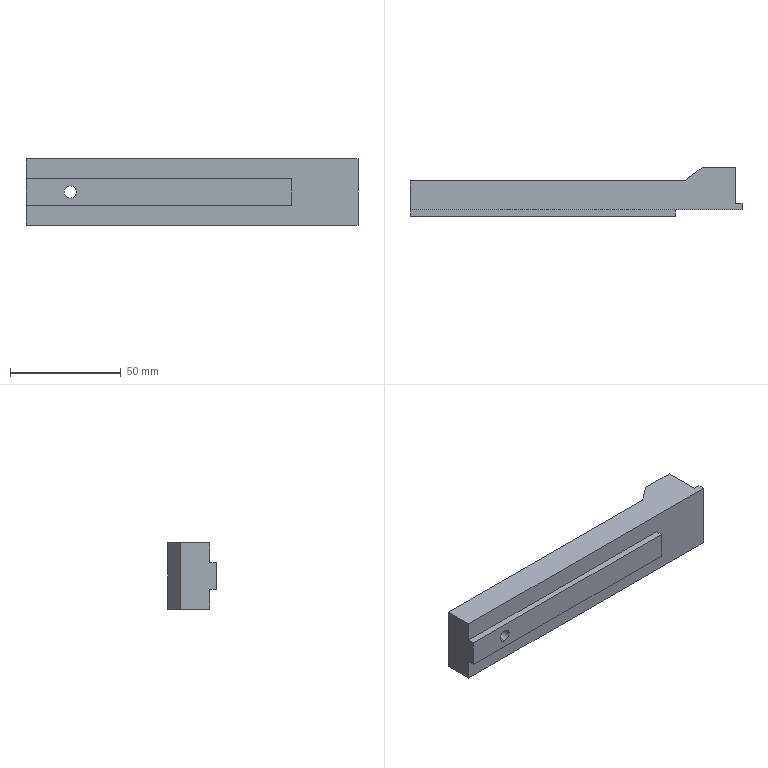Part | NX | features BREP 1 | 1 solid | 24 faces | box 150 x 22 x 30 mm | volume 64781 mm3 | plane 14 | cylinder 6 | cone 4 | commonest cylinder face diameters 3.3 x4 5.5 x2
STEP:
#1=CARTESIAN_POINT('',(132.,0.,15.));
#2=VERTEX_POINT('',#1);
#3=CARTESIAN_POINT('',(124.,-6.,15.));
#4=VERTEX_POINT('',#3);
#5=CARTESIAN_POINT('',(47.52,-63.36,15.));
#6=DIRECTION('',(-0.8,-0.6,0.));
#7=VECTOR('',#6,1000.);
#8=LINE('',#5,#7);
#9=EDGE_CURVE('',#2,#4,#8,.T.);
#10=ORIENTED_EDGE('',*,*,#9,.F.);
#11=CARTESIAN_POINT('',(132.,0.,-15.));
#12=VERTEX_POINT('',#11);
#13=CARTESIAN_POINT('',(132.,0.,-15.));
#14=DIRECTION('',(0.,0.,1.));
#15=VECTOR('',#14,1000.);
#16=LINE('',#13,#15);
#17=EDGE_CURVE('',#12,#2,#16,.T.);
#18=ORIENTED_EDGE('',*,*,#17,.F.);
#19=CARTESIAN_POINT('',(124.,-6.,-15.));
#20=VERTEX_POINT('',#19);
#21=CARTESIAN_POINT('',(47.52,-63.36,-15.));
#22=DIRECTION('',(-0.8,-0.6,0.));
#23=VECTOR('',#22,1000.);
#24=LINE('',#21,#23);
#25=EDGE_CURVE('',#12,#20,#24,.T.);
#26=ORIENTED_EDGE('',*,*,#25,.T.);
#27=CARTESIAN_POINT('',(124.,-6.,-15.));
#28=DIRECTION('',(0.,0.,1.));
#29=VECTOR('',#28,1000.);
#30=LINE('',#27,#29);
#31=EDGE_CURVE('',#20,#4,#30,.T.);
#32=ORIENTED_EDGE('',*,*,#31,.T.);
#33=EDGE_LOOP('',(#10,#18,#26,#32));
#34=FACE_BOUND('',#33,.T.);
#35=CARTESIAN_POINT('',(47.52,-63.36,-15.));
#36=DIRECTION('',(-0.6,0.8,0.));
#37=DIRECTION('',(-0.8,-0.6,0.));
#38=AXIS2_PLACEMENT_3D('',#35,#36,#37);
#39=PLANE('',#38);
#40=ADVANCED_FACE('',(#34),#39,.T.);
#41=CARTESIAN_POINT('',(20.,-6.,2.75));
#42=VERTEX_POINT('',#41);
#43=CARTESIAN_POINT('',(20.,-6.,-2.75));
#44=VERTEX_POINT('',#43);
#45=CARTESIAN_POINT('',(20.,-6.,0.));
#46=DIRECTION('',(0.,1.,0.));
#47=DIRECTION('',(0.,0.,-1.));
#48=AXIS2_PLACEMENT_3D('',#45,#46,#47);
#49=CIRCLE('',#48,2.75);
#50=EDGE_CURVE('',#42,#44,#49,.T.);
#51=ORIENTED_EDGE('',*,*,#50,.F.);
#52=CARTESIAN_POINT('',(20.,-6.,0.));
#53=DIRECTION('',(0.,1.,0.));
#54=DIRECTION('',(0.,0.,-1.));
#55=AXIS2_PLACEMENT_3D('',#52,#53,#54);
#56=CIRCLE('',#55,2.75);
#57=EDGE_CURVE('',#44,#42,#56,.T.);
#58=ORIENTED_EDGE('',*,*,#57,.F.);
#59=EDGE_LOOP('',(#51,#58));
#60=FACE_BOUND('',#59,.T.);
#61=CARTESIAN_POINT('',(0.,-6.,15.));
#62=VERTEX_POINT('',#61);
#63=CARTESIAN_POINT('',(0.,-6.,15.));
#64=DIRECTION('',(1.,0.,0.));
#65=VECTOR('',#64,1000.);
#66=LINE('',#63,#65);
#67=EDGE_CURVE('',#62,#4,#66,.T.);
#68=ORIENTED_EDGE('',*,*,#67,.T.);
#69=ORIENTED_EDGE('',*,*,#31,.F.);
#70=CARTESIAN_POINT('',(0.,-6.,-15.));
#71=VERTEX_POINT('',#70);
#72=CARTESIAN_POINT('',(0.,-6.,-15.));
#73=DIRECTION('',(1.,0.,0.));
#74=VECTOR('',#73,1000.);
#75=LINE('',#72,#74);
#76=EDGE_CURVE('',#71,#20,#75,.T.);
#77=ORIENTED_EDGE('',*,*,#76,.F.);
#78=CARTESIAN_POINT('',(0.,-6.,-15.));
#79=DIRECTION('',(0.,0.,1.));
#80=VECTOR('',#79,1000.);
#81=LINE('',#78,#80);
#82=EDGE_CURVE('',#71,#62,#81,.T.);
#83=ORIENTED_EDGE('',*,*,#82,.T.);
#84=EDGE_LOOP('',(#68,#69,#77,#83));
#85=FACE_BOUND('',#84,.T.);
#86=CARTESIAN_POINT('',(0.,-6.,-15.));
#87=DIRECTION('',(0.,-1.,0.));
#88=DIRECTION('',(0.,0.,-1.));
#89=AXIS2_PLACEMENT_3D('',#86,#87,#88);
#90=PLANE('',#89);
#91=ADVANCED_FACE('',(#60,#85),#90,.F.);
#92=CARTESIAN_POINT('',(20.,-22.,-2.75));
#93=VERTEX_POINT('',#92);
#94=CARTESIAN_POINT('',(20.,0.,-2.75));
#95=DIRECTION('',(0.,1.,0.));
#96=VECTOR('',#95,1000.);
#97=LINE('',#94,#96);
#98=EDGE_CURVE('',#44,#93,#97,.F.);
#99=ORIENTED_EDGE('',*,*,#98,.T.);
#100=CARTESIAN_POINT('',(20.,-22.,2.75));
#101=VERTEX_POINT('',#100);
#102=CARTESIAN_POINT('',(20.,-22.,0.));
#103=DIRECTION('',(0.,1.,0.));
#104=DIRECTION('',(0.,0.,1.));
#105=AXIS2_PLACEMENT_3D('',#102,#103,#104);
#106=CIRCLE('',#105,2.75);
#107=EDGE_CURVE('',#101,#93,#106,.T.);
#108=ORIENTED_EDGE('',*,*,#107,.F.);
#109=CARTESIAN_POINT('',(20.,0.,2.75));
#110=DIRECTION('',(0.,1.,0.));
#111=VECTOR('',#110,1000.);
#112=LINE('',#109,#111);
#113=EDGE_CURVE('',#42,#101,#112,.F.);
#114=ORIENTED_EDGE('',*,*,#113,.F.);
#115=ORIENTED_EDGE('',*,*,#50,.T.);
#116=EDGE_LOOP('',(#99,#108,#114,#115));
#117=FACE_BOUND('',#116,.T.);
#118=CARTESIAN_POINT('',(20.,0.,0.));
#119=DIRECTION('',(0.,1.,0.));
#120=DIRECTION('',(0.,0.,1.));
#121=AXIS2_PLACEMENT_3D('',#118,#119,#120);
#122=CYLINDRICAL_SURFACE('',#121,2.75);
#123=ADVANCED_FACE('',(#117),#122,.F.);
#124=CARTESIAN_POINT('',(136.9,-9.5,9.15));
#125=VERTEX_POINT('',#124);
#126=CARTESIAN_POINT('',(147.,-9.5,9.15));
#127=VERTEX_POINT('',#126);
#128=CARTESIAN_POINT('',(147.,-9.5,9.15));
#129=DIRECTION('',(1.,0.,0.));
#130=VECTOR('',#129,1000.);
#131=LINE('',#128,#130);
#132=EDGE_CURVE('',#125,#127,#131,.T.);
#133=ORIENTED_EDGE('',*,*,#132,.F.);
#134=CARTESIAN_POINT('',(136.9,-9.5,5.85));
#135=VERTEX_POINT('',#134);
#136=CARTESIAN_POINT('',(136.9,-9.5,7.5));
#137=DIRECTION('',(1.,0.,0.));
#138=DIRECTION('',(0.,0.,-1.));
#139=AXIS2_PLACEMENT_3D('',#136,#137,#138);
#140=CIRCLE('',#139,1.65);
#141=EDGE_CURVE('',#135,#125,#140,.T.);
#142=ORIENTED_EDGE('',*,*,#141,.F.);
#143=CARTESIAN_POINT('',(147.,-9.5,5.85));
#144=VERTEX_POINT('',#143);
#145=CARTESIAN_POINT('',(147.,-9.5,5.85));
#146=DIRECTION('',(1.,0.,0.));
#147=VECTOR('',#146,1000.);
#148=LINE('',#145,#147);
#149=EDGE_CURVE('',#135,#144,#148,.T.);
#150=ORIENTED_EDGE('',*,*,#149,.T.);
#151=CARTESIAN_POINT('',(147.,-9.5,7.5));
#152=DIRECTION('',(1.,0.,0.));
#153=DIRECTION('',(0.,0.,-1.));
#154=AXIS2_PLACEMENT_3D('',#151,#152,#153);
#155=CIRCLE('',#154,1.65);
#156=EDGE_CURVE('',#144,#127,#155,.T.);
#157=ORIENTED_EDGE('',*,*,#156,.T.);
#158=EDGE_LOOP('',(#133,#142,#150,#157));
#159=FACE_BOUND('',#158,.T.);
#160=CARTESIAN_POINT('',(147.,-9.5,7.5));
#161=DIRECTION('',(1.,0.,0.));
#162=DIRECTION('',(0.,0.,-1.));
#163=AXIS2_PLACEMENT_3D('',#160,#161,#162);
#164=CYLINDRICAL_SURFACE('',#163,1.65);
#165=ADVANCED_FACE('',(#159),#164,.F.);
#166=CARTESIAN_POINT('',(135.909,-9.5,7.5));
#167=VERTEX_POINT('',#166);
#168=CARTESIAN_POINT('',(136.9,-9.5,9.15));
#169=DIRECTION('',(0.515,0.,0.8572));
#170=VECTOR('',#169,1000.);
#171=LINE('',#168,#170);
#172=EDGE_CURVE('',#125,#167,#171,.F.);
#173=ORIENTED_EDGE('',*,*,#172,.T.);
#174=CARTESIAN_POINT('',(136.9,-9.5,5.85));
#175=DIRECTION('',(0.515,0.,-0.8572));
#176=VECTOR('',#175,1000.);
#177=LINE('',#174,#176);
#178=EDGE_CURVE('',#135,#167,#177,.F.);
#179=ORIENTED_EDGE('',*,*,#178,.F.);
#180=ORIENTED_EDGE('',*,*,#141,.T.);
#181=EDGE_LOOP('',(#173,#179,#180));
#182=FACE_BOUND('',#181,.T.);
#183=CARTESIAN_POINT('',(136.9,-9.5,7.5));
#184=DIRECTION('',(1.,0.,0.));
#185=DIRECTION('',(0.,0.,-1.));
#186=AXIS2_PLACEMENT_3D('',#183,#184,#185);
#187=CONICAL_SURFACE('',#186,1.65,1.03);
#188=ADVANCED_FACE('',(#182),#187,.F.);
#189=CARTESIAN_POINT('',(136.9,-9.5,-5.85));
#190=VERTEX_POINT('',#189);
#191=CARTESIAN_POINT('',(147.,-9.5,-5.85));
#192=VERTEX_POINT('',#191);
#193=CARTESIAN_POINT('',(147.,-9.5,-5.85));
#194=DIRECTION('',(1.,0.,0.));
#195=VECTOR('',#194,1000.);
#196=LINE('',#193,#195);
#197=EDGE_CURVE('',#190,#192,#196,.T.);
#198=ORIENTED_EDGE('',*,*,#197,.F.);
#199=CARTESIAN_POINT('',(136.9,-9.5,-9.15));
#200=VERTEX_POINT('',#199);
#201=CARTESIAN_POINT('',(136.9,-9.5,-7.5));
#202=DIRECTION('',(1.,0.,0.));
#203=DIRECTION('',(0.,0.,-1.));
#204=AXIS2_PLACEMENT_3D('',#201,#202,#203);
#205=CIRCLE('',#204,1.65);
#206=EDGE_CURVE('',#200,#190,#205,.T.);
#207=ORIENTED_EDGE('',*,*,#206,.F.);
#208=CARTESIAN_POINT('',(147.,-9.5,-9.15));
#209=VERTEX_POINT('',#208);
#210=CARTESIAN_POINT('',(147.,-9.5,-9.15));
#211=DIRECTION('',(1.,0.,0.));
#212=VECTOR('',#211,1000.);
#213=LINE('',#210,#212);
#214=EDGE_CURVE('',#200,#209,#213,.T.);
#215=ORIENTED_EDGE('',*,*,#214,.T.);
#216=CARTESIAN_POINT('',(147.,-9.5,-7.5));
#217=DIRECTION('',(1.,0.,0.));
#218=DIRECTION('',(0.,0.,-1.));
#219=AXIS2_PLACEMENT_3D('',#216,#217,#218);
#220=CIRCLE('',#219,1.65);
#221=EDGE_CURVE('',#209,#192,#220,.T.);
#222=ORIENTED_EDGE('',*,*,#221,.T.);
#223=EDGE_LOOP('',(#198,#207,#215,#222));
#224=FACE_BOUND('',#223,.T.);
#225=CARTESIAN_POINT('',(147.,-9.5,-7.5));
#226=DIRECTION('',(1.,0.,0.));
#227=DIRECTION('',(0.,0.,-1.));
#228=AXIS2_PLACEMENT_3D('',#225,#226,#227);
#229=CYLINDRICAL_SURFACE('',#228,1.65);
#230=ADVANCED_FACE('',(#224),#229,.F.);
#231=CARTESIAN_POINT('',(135.909,-9.5,-7.5));
#232=VERTEX_POINT('',#231);
#233=CARTESIAN_POINT('',(136.9,-9.5,-5.85));
#234=DIRECTION('',(0.515,0.,0.8572));
#235=VECTOR('',#234,1000.);
#236=LINE('',#233,#235);
#237=EDGE_CURVE('',#190,#232,#236,.F.);
#238=ORIENTED_EDGE('',*,*,#237,.T.);
#239=CARTESIAN_POINT('',(136.9,-9.5,-9.15));
#240=DIRECTION('',(0.515,0.,-0.8572));
#241=VECTOR('',#240,1000.);
#242=LINE('',#239,#241);
#243=EDGE_CURVE('',#200,#232,#242,.F.);
#244=ORIENTED_EDGE('',*,*,#243,.F.);
#245=ORIENTED_EDGE('',*,*,#206,.T.);
#246=EDGE_LOOP('',(#238,#244,#245));
#247=FACE_BOUND('',#246,.T.);
#248=CARTESIAN_POINT('',(136.9,-9.5,-7.5));
#249=DIRECTION('',(1.,0.,0.));
#250=DIRECTION('',(0.,0.,-1.));
#251=AXIS2_PLACEMENT_3D('',#248,#249,#250);
#252=CONICAL_SURFACE('',#251,1.65,1.03);
#253=ADVANCED_FACE('',(#247),#252,.F.);
#254=CARTESIAN_POINT('',(0.,-22.,6.));
#255=VERTEX_POINT('',#254);
#256=CARTESIAN_POINT('',(0.,-22.,-6.));
#257=VERTEX_POINT('',#256);
#258=CARTESIAN_POINT('',(0.,-22.,-6.));
#259=DIRECTION('',(0.,0.,-1.));
#260=VECTOR('',#259,1000.);
#261=LINE('',#258,#260);
#262=EDGE_CURVE('',#255,#257,#261,.T.);
#263=ORIENTED_EDGE('',*,*,#262,.T.);
#264=CARTESIAN_POINT('',(120.,-22.,-6.));
#265=VERTEX_POINT('',#264);
#266=CARTESIAN_POINT('',(120.,-22.,-6.));
#267=DIRECTION('',(1.,0.,0.));
#268=VECTOR('',#267,1000.);
#269=LINE('',#266,#268);
#270=EDGE_CURVE('',#257,#265,#269,.T.);
#271=ORIENTED_EDGE('',*,*,#270,.T.);
#272=CARTESIAN_POINT('',(120.,-22.,6.));
#273=VERTEX_POINT('',#272);
#274=CARTESIAN_POINT('',(120.,-22.,-6.));
#275=DIRECTION('',(0.,0.,1.));
#276=VECTOR('',#275,1000.);
#277=LINE('',#274,#276);
#278=EDGE_CURVE('',#265,#273,#277,.T.);
#279=ORIENTED_EDGE('',*,*,#278,.T.);
#280=CARTESIAN_POINT('',(120.,-22.,6.));
#281=DIRECTION('',(-1.,0.,0.));
#282=VECTOR('',#281,1000.);
#283=LINE('',#280,#282);
#284=EDGE_CURVE('',#273,#255,#283,.T.);
#285=ORIENTED_EDGE('',*,*,#284,.T.);
#286=EDGE_LOOP('',(#263,#271,#279,#285));
#287=FACE_BOUND('',#286,.T.);
#288=ORIENTED_EDGE('',*,*,#107,.T.);
#289=CARTESIAN_POINT('',(20.,-22.,0.));
#290=DIRECTION('',(0.,1.,0.));
#291=DIRECTION('',(0.,0.,1.));
#292=AXIS2_PLACEMENT_3D('',#289,#290,#291);
#293=CIRCLE('',#292,2.75);
#294=EDGE_CURVE('',#93,#101,#293,.T.);
#295=ORIENTED_EDGE('',*,*,#294,.T.);
#296=EDGE_LOOP('',(#288,#295));
#297=FACE_BOUND('',#296,.T.);
#298=CARTESIAN_POINT('',(0.,-22.,0.));
#299=DIRECTION('',(0.,-1.,0.));
#300=DIRECTION('',(1.,0.,0.));
#301=AXIS2_PLACEMENT_3D('',#298,#299,#300);
#302=PLANE('',#301);
#303=ADVANCED_FACE('',(#287,#297),#302,.T.);
#304=CARTESIAN_POINT('',(120.,-19.,6.));
#305=VERTEX_POINT('',#304);
#306=CARTESIAN_POINT('',(0.,-19.,6.));
#307=VERTEX_POINT('',#306);
#308=CARTESIAN_POINT('',(120.,-19.,6.));
#309=DIRECTION('',(-1.,0.,0.));
#310=VECTOR('',#309,1000.);
#311=LINE('',#308,#310);
#312=EDGE_CURVE('',#305,#307,#311,.T.);
#313=ORIENTED_EDGE('',*,*,#312,.T.);
#314=CARTESIAN_POINT('',(0.,-22.,6.));
#315=DIRECTION('',(0.,1.,0.));
#316=VECTOR('',#315,1000.);
#317=LINE('',#314,#316);
#318=EDGE_CURVE('',#255,#307,#317,.T.);
#319=ORIENTED_EDGE('',*,*,#318,.F.);
#320=ORIENTED_EDGE('',*,*,#284,.F.);
#321=CARTESIAN_POINT('',(120.,-22.,6.));
#322=DIRECTION('',(0.,1.,0.));
#323=VECTOR('',#322,1000.);
#324=LINE('',#321,#323);
#325=EDGE_CURVE('',#273,#305,#324,.T.);
#326=ORIENTED_EDGE('',*,*,#325,.T.);
#327=EDGE_LOOP('',(#313,#319,#320,#326));
#328=FACE_BOUND('',#327,.T.);
#329=CARTESIAN_POINT('',(120.,-22.,6.));
#330=DIRECTION('',(0.,0.,-1.));
#331=DIRECTION('',(-1.,0.,0.));
#332=AXIS2_PLACEMENT_3D('',#329,#330,#331);
#333=PLANE('',#332);
#334=ADVANCED_FACE('',(#328),#333,.F.);
#335=CARTESIAN_POINT('',(120.,-19.,-6.));
#336=VERTEX_POINT('',#335);
#337=CARTESIAN_POINT('',(120.,-19.,-6.));
#338=DIRECTION('',(0.,0.,1.));
#339=VECTOR('',#338,1000.);
#340=LINE('',#337,#339);
#341=EDGE_CURVE('',#336,#305,#340,.T.);
#342=ORIENTED_EDGE('',*,*,#341,.T.);
#343=ORIENTED_EDGE('',*,*,#325,.F.);
#344=ORIENTED_EDGE('',*,*,#278,.F.);
#345=CARTESIAN_POINT('',(120.,-22.,-6.));
#346=DIRECTION('',(0.,1.,0.));
#347=VECTOR('',#346,1000.);
#348=LINE('',#345,#347);
#349=EDGE_CURVE('',#265,#336,#348,.T.);
#350=ORIENTED_EDGE('',*,*,#349,.T.);
#351=EDGE_LOOP('',(#342,#343,#344,#350));
#352=FACE_BOUND('',#351,.T.);
#353=CARTESIAN_POINT('',(120.,-22.,-6.));
#354=DIRECTION('',(-1.,0.,0.));
#355=DIRECTION('',(0.,-1.,0.));
#356=AXIS2_PLACEMENT_3D('',#353,#354,#355);
#357=PLANE('',#356);
#358=ADVANCED_FACE('',(#352),#357,.F.);
#359=CARTESIAN_POINT('',(0.,-19.,-6.));
#360=VERTEX_POINT('',#359);
#361=CARTESIAN_POINT('',(120.,-19.,-6.));
#362=DIRECTION('',(1.,0.,0.));
#363=VECTOR('',#362,1000.);
#364=LINE('',#361,#363);
#365=EDGE_CURVE('',#360,#336,#364,.T.);
#366=ORIENTED_EDGE('',*,*,#365,.T.);
#367=ORIENTED_EDGE('',*,*,#349,.F.);
#368=ORIENTED_EDGE('',*,*,#270,.F.);
#369=CARTESIAN_POINT('',(0.,-22.,-6.));
#370=DIRECTION('',(0.,1.,0.));
#371=VECTOR('',#370,1000.);
#372=LINE('',#369,#371);
#373=EDGE_CURVE('',#257,#360,#372,.T.);
#374=ORIENTED_EDGE('',*,*,#373,.T.);
#375=EDGE_LOOP('',(#366,#367,#368,#374));
#376=FACE_BOUND('',#375,.T.);
#377=CARTESIAN_POINT('',(120.,-22.,-6.));
#378=DIRECTION('',(0.,0.,1.));
#379=DIRECTION('',(1.,0.,0.));
#380=AXIS2_PLACEMENT_3D('',#377,#378,#379);
#381=PLANE('',#380);
#382=ADVANCED_FACE('',(#376),#381,.F.);
#383=CARTESIAN_POINT('',(150.,-16.,-15.));
#384=VERTEX_POINT('',#383);
#385=CARTESIAN_POINT('',(147.,-16.,-15.));
#386=VERTEX_POINT('',#385);
#387=CARTESIAN_POINT('',(147.,-16.,-15.));
#388=DIRECTION('',(-1.,0.,0.));
#389=VECTOR('',#388,1000.);
#390=LINE('',#387,#389);
#391=EDGE_CURVE('',#384,#386,#390,.T.);
#392=ORIENTED_EDGE('',*,*,#391,.T.);
#393=CARTESIAN_POINT('',(147.,-16.,15.));
#394=VERTEX_POINT('',#393);
#395=CARTESIAN_POINT('',(147.,-16.,15.));
#396=DIRECTION('',(0.,0.,-1.));
#397=VECTOR('',#396,1000.);
#398=LINE('',#395,#397);
#399=EDGE_CURVE('',#394,#386,#398,.T.);
#400=ORIENTED_EDGE('',*,*,#399,.F.);
#401=CARTESIAN_POINT('',(150.,-16.,15.));
#402=VERTEX_POINT('',#401);
#403=CARTESIAN_POINT('',(147.,-16.,15.));
#404=DIRECTION('',(-1.,0.,0.));
#405=VECTOR('',#404,1000.);
#406=LINE('',#403,#405);
#407=EDGE_CURVE('',#402,#394,#406,.T.);
#408=ORIENTED_EDGE('',*,*,#407,.F.);
#409=CARTESIAN_POINT('',(150.,-16.,15.));
#410=DIRECTION('',(0.,0.,-1.));
#411=VECTOR('',#410,1000.);
#412=LINE('',#409,#411);
#413=EDGE_CURVE('',#402,#384,#412,.T.);
#414=ORIENTED_EDGE('',*,*,#413,.T.);
#415=EDGE_LOOP('',(#392,#400,#408,#414));
#416=FACE_BOUND('',#415,.T.);
#417=CARTESIAN_POINT('',(147.,-16.,15.));
#418=DIRECTION('',(0.,-1.,0.));
#419=DIRECTION('',(0.,0.,-1.));
#420=AXIS2_PLACEMENT_3D('',#417,#418,#419);
#421=PLANE('',#420);
#422=ADVANCED_FACE('',(#416),#421,.F.);
#423=CARTESIAN_POINT('',(150.,-19.,-15.));
#424=VERTEX_POINT('',#423);
#425=CARTESIAN_POINT('',(150.,-16.,-15.));
#426=DIRECTION('',(0.,1.,0.));
#427=VECTOR('',#426,1000.);
#428=LINE('',#425,#427);
#429=EDGE_CURVE('',#424,#384,#428,.T.);
#430=ORIENTED_EDGE('',*,*,#429,.T.);
#431=ORIENTED_EDGE('',*,*,#413,.F.);
#432=CARTESIAN_POINT('',(150.,-19.,15.));
#433=VERTEX_POINT('',#432);
#434=CARTESIAN_POINT('',(150.,-16.,15.));
#435=DIRECTION('',(0.,1.,0.));
#436=VECTOR('',#435,1000.);
#437=LINE('',#434,#436);
#438=EDGE_CURVE('',#433,#402,#437,.T.);
#439=ORIENTED_EDGE('',*,*,#438,.F.);
#440=CARTESIAN_POINT('',(150.,-19.,15.));
#441=DIRECTION('',(0.,0.,-1.));
#442=VECTOR('',#441,1000.);
#443=LINE('',#440,#442);
#444=EDGE_CURVE('',#433,#424,#443,.T.);
#445=ORIENTED_EDGE('',*,*,#444,.T.);
#446=EDGE_LOOP('',(#430,#431,#439,#445));
#447=FACE_BOUND('',#446,.T.);
#448=CARTESIAN_POINT('',(150.,-16.,15.));
#449=DIRECTION('',(-1.,0.,0.));
#450=DIRECTION('',(0.,0.,1.));
#451=AXIS2_PLACEMENT_3D('',#448,#449,#450);
#452=PLANE('',#451);
#453=ADVANCED_FACE('',(#447),#452,.F.);
#454=CARTESIAN_POINT('',(0.,-19.,15.));
#455=VERTEX_POINT('',#454);
#456=CARTESIAN_POINT('',(0.,0.,15.));
#457=DIRECTION('',(0.,-1.,0.));
#458=VECTOR('',#457,1000.);
#459=LINE('',#456,#458);
#460=EDGE_CURVE('',#62,#455,#459,.T.);
#461=ORIENTED_EDGE('',*,*,#460,.F.);
#462=ORIENTED_EDGE('',*,*,#82,.F.);
#463=CARTESIAN_POINT('',(0.,-19.,-15.));
#464=VERTEX_POINT('',#463);
#465=CARTESIAN_POINT('',(0.,0.,-15.));
#466=DIRECTION('',(0.,-1.,0.));
#467=VECTOR('',#466,1000.);
#468=LINE('',#465,#467);
#469=EDGE_CURVE('',#71,#464,#468,.T.);
#470=ORIENTED_EDGE('',*,*,#469,.T.);
#471=CARTESIAN_POINT('',(0.,-19.,15.));
#472=DIRECTION('',(0.,0.,-1.));
#473=VECTOR('',#472,1000.);
#474=LINE('',#471,#473);
#475=EDGE_CURVE('',#360,#464,#474,.T.);
#476=ORIENTED_EDGE('',*,*,#475,.F.);
#477=ORIENTED_EDGE('',*,*,#373,.F.);
#478=ORIENTED_EDGE('',*,*,#262,.F.);
#479=ORIENTED_EDGE('',*,*,#318,.T.);
#480=CARTESIAN_POINT('',(0.,-19.,15.));
#481=DIRECTION('',(0.,0.,-1.));
#482=VECTOR('',#481,1000.);
#483=LINE('',#480,#482);
#484=EDGE_CURVE('',#455,#307,#483,.T.);
#485=ORIENTED_EDGE('',*,*,#484,.F.);
#486=EDGE_LOOP('',(#461,#462,#470,#476,#477,#478,#479,#485));
#487=FACE_BOUND('',#486,.T.);
#488=CARTESIAN_POINT('',(0.,0.,15.));
#489=DIRECTION('',(1.,0.,0.));
#490=DIRECTION('',(0.,0.,-1.));
#491=AXIS2_PLACEMENT_3D('',#488,#489,#490);
#492=PLANE('',#491);
#493=ADVANCED_FACE('',(#487),#492,.F.);
#494=CARTESIAN_POINT('',(147.,0.,-15.));
#495=VERTEX_POINT('',#494);
#496=CARTESIAN_POINT('',(147.,0.,-15.));
#497=DIRECTION('',(0.,1.,0.));
#498=VECTOR('',#497,1000.);
#499=LINE('',#496,#498);
#500=EDGE_CURVE('',#386,#495,#499,.T.);
#501=ORIENTED_EDGE('',*,*,#500,.T.);
#502=CARTESIAN_POINT('',(147.,0.,15.));
#503=VERTEX_POINT('',#502);
#504=CARTESIAN_POINT('',(147.,0.,15.));
#505=DIRECTION('',(0.,0.,-1.));
#506=VECTOR('',#505,1000.);
#507=LINE('',#504,#506);
#508=EDGE_CURVE('',#503,#495,#507,.T.);
#509=ORIENTED_EDGE('',*,*,#508,.F.);
#510=CARTESIAN_POINT('',(147.,0.,15.));
#511=DIRECTION('',(0.,1.,0.));
#512=VECTOR('',#511,1000.);
#513=LINE('',#510,#512);
#514=EDGE_CURVE('',#394,#503,#513,.T.);
#515=ORIENTED_EDGE('',*,*,#514,.F.);
#516=ORIENTED_EDGE('',*,*,#399,.T.);
#517=EDGE_LOOP('',(#501,#509,#515,#516));
#518=FACE_BOUND('',#517,.T.);
#519=ORIENTED_EDGE('',*,*,#221,.F.);
#520=CARTESIAN_POINT('',(147.,-9.5,-7.5));
#521=DIRECTION('',(1.,0.,0.));
#522=DIRECTION('',(0.,0.,-1.));
#523=AXIS2_PLACEMENT_3D('',#520,#521,#522);
#524=CIRCLE('',#523,1.65);
#525=EDGE_CURVE('',#192,#209,#524,.T.);
#526=ORIENTED_EDGE('',*,*,#525,.F.);
#527=EDGE_LOOP('',(#519,#526));
#528=FACE_BOUND('',#527,.T.);
#529=ORIENTED_EDGE('',*,*,#156,.F.);
#530=CARTESIAN_POINT('',(147.,-9.5,7.5));
#531=DIRECTION('',(1.,0.,0.));
#532=DIRECTION('',(0.,0.,-1.));
#533=AXIS2_PLACEMENT_3D('',#530,#531,#532);
#534=CIRCLE('',#533,1.65);
#535=EDGE_CURVE('',#127,#144,#534,.T.);
#536=ORIENTED_EDGE('',*,*,#535,.F.);
#537=EDGE_LOOP('',(#529,#536));
#538=FACE_BOUND('',#537,.T.);
#539=CARTESIAN_POINT('',(147.,0.,15.));
#540=DIRECTION('',(-1.,0.,0.));
#541=DIRECTION('',(0.,0.,1.));
#542=AXIS2_PLACEMENT_3D('',#539,#540,#541);
#543=PLANE('',#542);
#544=ADVANCED_FACE('',(#518,#528,#538),#543,.F.);
#545=ORIENTED_EDGE('',*,*,#312,.F.);
#546=ORIENTED_EDGE('',*,*,#341,.F.);
#547=ORIENTED_EDGE('',*,*,#365,.F.);
#548=ORIENTED_EDGE('',*,*,#475,.T.);
#549=CARTESIAN_POINT('',(150.,-19.,-15.));
#550=DIRECTION('',(1.,0.,0.));
#551=VECTOR('',#550,1000.);
#552=LINE('',#549,#551);
#553=EDGE_CURVE('',#464,#424,#552,.T.);
#554=ORIENTED_EDGE('',*,*,#553,.T.);
#555=ORIENTED_EDGE('',*,*,#444,.F.);
#556=CARTESIAN_POINT('',(150.,-19.,15.));
#557=DIRECTION('',(1.,0.,0.));
#558=VECTOR('',#557,1000.);
#559=LINE('',#556,#558);
#560=EDGE_CURVE('',#455,#433,#559,.T.);
#561=ORIENTED_EDGE('',*,*,#560,.F.);
#562=ORIENTED_EDGE('',*,*,#484,.T.);
#563=EDGE_LOOP('',(#545,#546,#547,#548,#554,#555,#561,#562));
#564=FACE_BOUND('',#563,.T.);
#565=CARTESIAN_POINT('',(150.,-19.,15.));
#566=DIRECTION('',(0.,1.,0.));
#567=DIRECTION('',(-1.,0.,0.));
#568=AXIS2_PLACEMENT_3D('',#565,#566,#567);
#569=PLANE('',#568);
#570=ADVANCED_FACE('',(#564),#569,.F.);
#571=ORIENTED_EDGE('',*,*,#25,.F.);
#572=CARTESIAN_POINT('',(147.,0.,-15.));
#573=DIRECTION('',(-1.,0.,0.));
#574=VECTOR('',#573,1000.);
#575=LINE('',#572,#574);
#576=EDGE_CURVE('',#495,#12,#575,.T.);
#577=ORIENTED_EDGE('',*,*,#576,.F.);
#578=ORIENTED_EDGE('',*,*,#500,.F.);
#579=ORIENTED_EDGE('',*,*,#391,.F.);
#580=ORIENTED_EDGE('',*,*,#429,.F.);
#581=ORIENTED_EDGE('',*,*,#553,.F.);
#582=ORIENTED_EDGE('',*,*,#469,.F.);
#583=ORIENTED_EDGE('',*,*,#76,.T.);
#584=EDGE_LOOP('',(#571,#577,#578,#579,#580,#581,#582,#583));
#585=FACE_BOUND('',#584,.T.);
#586=CARTESIAN_POINT('',(0.,0.,-15.));
#587=DIRECTION('',(0.,0.,1.));
#588=DIRECTION('',(1.,0.,0.));
#589=AXIS2_PLACEMENT_3D('',#586,#587,#588);
#590=PLANE('',#589);
#591=ADVANCED_FACE('',(#585),#590,.F.);
#592=CARTESIAN_POINT('',(147.,0.,15.));
#593=DIRECTION('',(-1.,0.,0.));
#594=VECTOR('',#593,1000.);
#595=LINE('',#592,#594);
#596=EDGE_CURVE('',#503,#2,#595,.T.);
#597=ORIENTED_EDGE('',*,*,#596,.T.);
#598=ORIENTED_EDGE('',*,*,#9,.T.);
#599=ORIENTED_EDGE('',*,*,#67,.F.);
#600=ORIENTED_EDGE('',*,*,#460,.T.);
#601=ORIENTED_EDGE('',*,*,#560,.T.);
#602=ORIENTED_EDGE('',*,*,#438,.T.);
#603=ORIENTED_EDGE('',*,*,#407,.T.);
#604=ORIENTED_EDGE('',*,*,#514,.T.);
#605=EDGE_LOOP('',(#597,#598,#599,#600,#601,#602,#603,#604));
#606=FACE_BOUND('',#605,.T.);
#607=CARTESIAN_POINT('',(0.,0.,15.));
#608=DIRECTION('',(0.,0.,1.));
#609=DIRECTION('',(1.,0.,0.));
#610=AXIS2_PLACEMENT_3D('',#607,#608,#609);
#611=PLANE('',#610);
#612=ADVANCED_FACE('',(#606),#611,.T.);
#613=ORIENTED_EDGE('',*,*,#17,.T.);
#614=ORIENTED_EDGE('',*,*,#596,.F.);
#615=ORIENTED_EDGE('',*,*,#508,.T.);
#616=ORIENTED_EDGE('',*,*,#576,.T.);
#617=EDGE_LOOP('',(#613,#614,#615,#616));
#618=FACE_BOUND('',#617,.T.);
#619=CARTESIAN_POINT('',(147.,0.,15.));
#620=DIRECTION('',(0.,-1.,0.));
#621=DIRECTION('',(0.,0.,-1.));
#622=AXIS2_PLACEMENT_3D('',#619,#620,#621);
#623=PLANE('',#622);
#624=ADVANCED_FACE('',(#618),#623,.F.);
#625=ORIENTED_EDGE('',*,*,#243,.T.);
#626=ORIENTED_EDGE('',*,*,#237,.F.);
#627=CARTESIAN_POINT('',(136.9,-9.5,-7.5));
#628=DIRECTION('',(1.,0.,0.));
#629=DIRECTION('',(0.,0.,-1.));
#630=AXIS2_PLACEMENT_3D('',#627,#628,#629);
#631=CIRCLE('',#630,1.65);
#632=EDGE_CURVE('',#190,#200,#631,.T.);
#633=ORIENTED_EDGE('',*,*,#632,.T.);
#634=EDGE_LOOP('',(#625,#626,#633));
#635=FACE_BOUND('',#634,.T.);
#636=CARTESIAN_POINT('',(136.9,-9.5,-7.5));
#637=DIRECTION('',(1.,0.,0.));
#638=DIRECTION('',(0.,0.,-1.));
#639=AXIS2_PLACEMENT_3D('',#636,#637,#638);
#640=CONICAL_SURFACE('',#639,1.65,1.03);
#641=ADVANCED_FACE('',(#635),#640,.F.);
#642=ORIENTED_EDGE('',*,*,#632,.F.);
#643=ORIENTED_EDGE('',*,*,#197,.T.);
#644=ORIENTED_EDGE('',*,*,#525,.T.);
#645=ORIENTED_EDGE('',*,*,#214,.F.);
#646=EDGE_LOOP('',(#642,#643,#644,#645));
#647=FACE_BOUND('',#646,.T.);
#648=CARTESIAN_POINT('',(147.,-9.5,-7.5));
#649=DIRECTION('',(1.,0.,0.));
#650=DIRECTION('',(0.,0.,-1.));
#651=AXIS2_PLACEMENT_3D('',#648,#649,#650);
#652=CYLINDRICAL_SURFACE('',#651,1.65);
#653=ADVANCED_FACE('',(#647),#652,.F.);
#654=ORIENTED_EDGE('',*,*,#178,.T.);
#655=ORIENTED_EDGE('',*,*,#172,.F.);
#656=CARTESIAN_POINT('',(136.9,-9.5,7.5));
#657=DIRECTION('',(1.,0.,0.));
#658=DIRECTION('',(0.,0.,-1.));
#659=AXIS2_PLACEMENT_3D('',#656,#657,#658);
#660=CIRCLE('',#659,1.65);
#661=EDGE_CURVE('',#125,#135,#660,.T.);
#662=ORIENTED_EDGE('',*,*,#661,.T.);
#663=EDGE_LOOP('',(#654,#655,#662));
#664=FACE_BOUND('',#663,.T.);
#665=CARTESIAN_POINT('',(136.9,-9.5,7.5));
#666=DIRECTION('',(1.,0.,0.));
#667=DIRECTION('',(0.,0.,-1.));
#668=AXIS2_PLACEMENT_3D('',#665,#666,#667);
#669=CONICAL_SURFACE('',#668,1.65,1.03);
#670=ADVANCED_FACE('',(#664),#669,.F.);
#671=ORIENTED_EDGE('',*,*,#661,.F.);
#672=ORIENTED_EDGE('',*,*,#132,.T.);
#673=ORIENTED_EDGE('',*,*,#535,.T.);
#674=ORIENTED_EDGE('',*,*,#149,.F.);
#675=EDGE_LOOP('',(#671,#672,#673,#674));
#676=FACE_BOUND('',#675,.T.);
#677=CARTESIAN_POINT('',(147.,-9.5,7.5));
#678=DIRECTION('',(1.,0.,0.));
#679=DIRECTION('',(0.,0.,-1.));
#680=AXIS2_PLACEMENT_3D('',#677,#678,#679);
#681=CYLINDRICAL_SURFACE('',#680,1.65);
#682=ADVANCED_FACE('',(#676),#681,.F.);
#683=ORIENTED_EDGE('',*,*,#294,.F.);
#684=ORIENTED_EDGE('',*,*,#98,.F.);
#685=ORIENTED_EDGE('',*,*,#57,.T.);
#686=ORIENTED_EDGE('',*,*,#113,.T.);
#687=EDGE_LOOP('',(#683,#684,#685,#686));
#688=FACE_BOUND('',#687,.T.);
#689=CARTESIAN_POINT('',(20.,0.,0.));
#690=DIRECTION('',(0.,1.,0.));
#691=DIRECTION('',(0.,0.,1.));
#692=AXIS2_PLACEMENT_3D('',#689,#690,#691);
#693=CYLINDRICAL_SURFACE('',#692,2.75);
#694=ADVANCED_FACE('',(#688),#693,.F.);
#695=CLOSED_SHELL('',(#40,#91,#123,#165,#188,#230,#253,#303,#334,#358,#382,#422,#453,#493,#544,#570,#591,#612,#624,#641,#653,#670,#682,#694));
#696=MANIFOLD_SOLID_BREP('',#695);
#697=(LENGTH_UNIT()NAMED_UNIT(*)SI_UNIT(.MILLI.,.METRE.));
#698=UNCERTAINTY_MEASURE_WITH_UNIT(LENGTH_MEASURE(0.00001),#697,'','');
#699=(NAMED_UNIT(*)PLANE_ANGLE_UNIT()SI_UNIT($,.RADIAN.));
#700=(NAMED_UNIT(*)SI_UNIT($,.STERADIAN.)SOLID_ANGLE_UNIT());
#701=(GEOMETRIC_REPRESENTATION_CONTEXT(3)GLOBAL_UNCERTAINTY_ASSIGNED_CONTEXT((#698))GLOBAL_UNIT_ASSIGNED_CONTEXT((#697,#699,#700))REPRESENTATION_CONTEXT('',''));
#702=ADVANCED_BREP_SHAPE_REPRESENTATION('',(#696),#701);